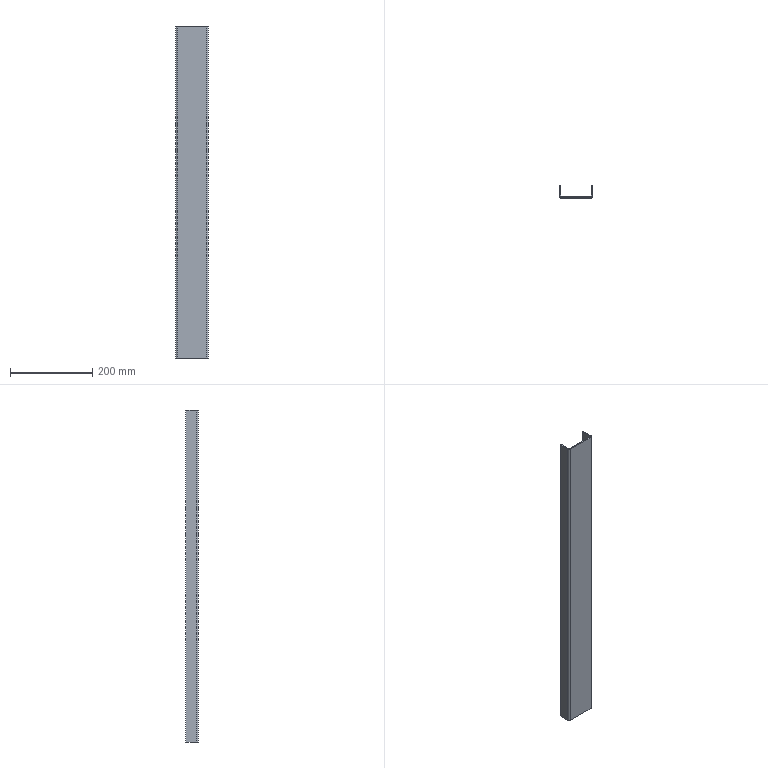Part | STEP file | Double-tube frame cross brace SGN-1-07 | 1 solid | 22 faces | box 80 x 30 x 807 mm | volume 318179 mm3 | plane 18 | cylinder 4 | commonest cylinder face diameters 3 x2 9 x2
STEP:
#1=CARTESIAN_POINT('',(0.,0.,0.));
#2=DIRECTION('',(0.,0.,1.));
#3=DIRECTION('',(1.,0.,0.));
#4=AXIS2_PLACEMENT_3D('',#1,#2,#3);
#5=CARTESIAN_POINT('',(35.5,-6.24,807.));
#6=VERTEX_POINT('',#5);
#7=CARTESIAN_POINT('',(35.5,-3.24,807.));
#8=VERTEX_POINT('',#7);
#9=CARTESIAN_POINT('',(35.5,-6.24,807.));
#10=DIRECTION('',(0.,1.,0.));
#11=VECTOR('',#10,1.);
#12=LINE('',#9,#11);
#13=CARTESIAN_POINT('',(35.5,-6.24,807.));
#14=DIRECTION('',(0.,0.,1.));
#15=DIRECTION('',(1.,0.,0.));
#16=AXIS2_PLACEMENT_3D('',#13,#14,#15);
#17=PLANE('',#16);
#18=CARTESIAN_POINT('',(0.,0.));
#19=DIRECTION('',(0.,1.));
#20=VECTOR('',#19,1.);
#21=LINE('',#18,#20);
#22=(GEOMETRIC_REPRESENTATION_CONTEXT(2)PARAMETRIC_REPRESENTATION_CONTEXT()REPRESENTATION_CONTEXT('',''));
#23=DEFINITIONAL_REPRESENTATION('',(#21),#22);
#24=PCURVE('',#17,#23);
#25=CARTESIAN_POINT('',(37.,-1.74,807.));
#26=DIRECTION('',(0.,0.,1.));
#27=DIRECTION('',(1.,0.,0.));
#28=AXIS2_PLACEMENT_3D('',#25,#26,#27);
#29=PLANE('',#28);
#30=CARTESIAN_POINT('',(-1.5,-4.5));
#31=DIRECTION('',(0.,1.));
#32=VECTOR('',#31,1.);
#33=LINE('',#30,#32);
#34=(GEOMETRIC_REPRESENTATION_CONTEXT(2)PARAMETRIC_REPRESENTATION_CONTEXT()REPRESENTATION_CONTEXT('',''));
#35=DEFINITIONAL_REPRESENTATION('',(#33),#34);
#36=PCURVE('',#29,#35);
#37=SURFACE_CURVE('',#12,(#24,#36),.PCURVE_S1.);
#38=EDGE_CURVE('',#6,#8,#37,.T.);
#39=ORIENTED_EDGE('',*,*,#38,.F.);
#40=CARTESIAN_POINT('',(40.,-1.74,807.));
#41=VERTEX_POINT('',#40);
#42=CARTESIAN_POINT('',(35.5,-1.74,807.));
#43=DIRECTION('',(0.,0.,-1.));
#44=DIRECTION('',(1.,0.,0.));
#45=AXIS2_PLACEMENT_3D('',#42,#43,#44);
#46=CIRCLE('',#45,4.5);
#47=CARTESIAN_POINT('',(4.5,4.5));
#48=CARTESIAN_POINT('',(4.5,-3.294));
#49=CARTESIAN_POINT('',(-2.25,0.6029));
#50=CARTESIAN_POINT('',(-9.,4.5));
#51=CARTESIAN_POINT('',(-2.25,8.397));
#52=CARTESIAN_POINT('',(4.5,12.294));
#53=CARTESIAN_POINT('',(4.5,4.5));
#54=(BOUNDED_CURVE()B_SPLINE_CURVE(2,(#47,#48,#49,#50,#51,#52,#53),.UNSPECIFIED.,.T.,.F.)B_SPLINE_CURVE_WITH_KNOTS((1,2,2,2,2,1),(-2.094,0.,2.094,4.189,6.283,8.378),.UNSPECIFIED.)CURVE()GEOMETRIC_REPRESENTATION_ITEM()RATIONAL_B_SPLINE_CURVE((1.,0.5,1.,0.5,1.,0.5,1.))REPRESENTATION_ITEM(''));
#55=(GEOMETRIC_REPRESENTATION_CONTEXT(2)PARAMETRIC_REPRESENTATION_CONTEXT()REPRESENTATION_CONTEXT('',''));
#56=DEFINITIONAL_REPRESENTATION('',(#54),#55);
#57=PCURVE('',#17,#56);
#58=CARTESIAN_POINT('',(35.5,-1.74,807.));
#59=DIRECTION('',(0.,0.,-1.));
#60=DIRECTION('',(-1.,0.,0.));
#61=AXIS2_PLACEMENT_3D('',#58,#59,#60);
#62=CYLINDRICAL_SURFACE('',#61,4.5);
#63=CARTESIAN_POINT('',(3.142,0.));
#64=DIRECTION('',(1.,0.));
#65=VECTOR('',#64,1.);
#66=LINE('',#63,#65);
#67=(GEOMETRIC_REPRESENTATION_CONTEXT(2)PARAMETRIC_REPRESENTATION_CONTEXT()REPRESENTATION_CONTEXT('',''));
#68=DEFINITIONAL_REPRESENTATION('',(#66),#67);
#69=PCURVE('',#62,#68);
#70=SURFACE_CURVE('',#46,(#57,#69),.PCURVE_S1.);
#71=EDGE_CURVE('',#41,#6,#70,.T.);
#72=ORIENTED_EDGE('',*,*,#71,.F.);
#73=CARTESIAN_POINT('',(37.,-1.74,807.));
#74=VERTEX_POINT('',#73);
#75=CARTESIAN_POINT('',(37.,-1.74,807.));
#76=DIRECTION('',(1.,0.,0.));
#77=VECTOR('',#76,1.);
#78=LINE('',#75,#77);
#79=CARTESIAN_POINT('',(1.5,4.5));
#80=DIRECTION('',(1.,0.));
#81=VECTOR('',#80,1.);
#82=LINE('',#79,#81);
#83=(GEOMETRIC_REPRESENTATION_CONTEXT(2)PARAMETRIC_REPRESENTATION_CONTEXT()REPRESENTATION_CONTEXT('',''));
#84=DEFINITIONAL_REPRESENTATION('',(#82),#83);
#85=PCURVE('',#17,#84);
#86=CARTESIAN_POINT('',(-35.5,-1.74,807.));
#87=DIRECTION('',(0.,0.,1.));
#88=DIRECTION('',(1.,0.,0.));
#89=AXIS2_PLACEMENT_3D('',#86,#87,#88);
#90=PLANE('',#89);
#91=CARTESIAN_POINT('',(72.5,0.));
#92=DIRECTION('',(1.,0.));
#93=VECTOR('',#92,1.);
#94=LINE('',#91,#93);
#95=(GEOMETRIC_REPRESENTATION_CONTEXT(2)PARAMETRIC_REPRESENTATION_CONTEXT()REPRESENTATION_CONTEXT('',''));
#96=DEFINITIONAL_REPRESENTATION('',(#94),#95);
#97=PCURVE('',#90,#96);
#98=SURFACE_CURVE('',#78,(#85,#97),.PCURVE_S1.);
#99=EDGE_CURVE('',#74,#41,#98,.T.);
#100=ORIENTED_EDGE('',*,*,#99,.F.);
#101=CARTESIAN_POINT('',(35.5,-1.74,807.));
#102=DIRECTION('',(0.,0.,-1.));
#103=DIRECTION('',(1.,0.,0.));
#104=AXIS2_PLACEMENT_3D('',#101,#102,#103);
#105=CIRCLE('',#104,1.5);
#106=CARTESIAN_POINT('',(1.5,4.5));
#107=CARTESIAN_POINT('',(1.5,1.902));
#108=CARTESIAN_POINT('',(-0.75,3.201));
#109=CARTESIAN_POINT('',(-3.,4.5));
#110=CARTESIAN_POINT('',(-0.75,5.799));
#111=CARTESIAN_POINT('',(1.5,7.098));
#112=CARTESIAN_POINT('',(1.5,4.5));
#113=(BOUNDED_CURVE()B_SPLINE_CURVE(2,(#106,#107,#108,#109,#110,#111,#112),.UNSPECIFIED.,.T.,.F.)B_SPLINE_CURVE_WITH_KNOTS((1,2,2,2,2,1),(-2.094,0.,2.094,4.189,6.283,8.378),.UNSPECIFIED.)CURVE()GEOMETRIC_REPRESENTATION_ITEM()RATIONAL_B_SPLINE_CURVE((1.,0.5,1.,0.5,1.,0.5,1.))REPRESENTATION_ITEM(''));
#114=(GEOMETRIC_REPRESENTATION_CONTEXT(2)PARAMETRIC_REPRESENTATION_CONTEXT()REPRESENTATION_CONTEXT('',''));
#115=DEFINITIONAL_REPRESENTATION('',(#113),#114);
#116=PCURVE('',#17,#115);
#117=CARTESIAN_POINT('',(35.5,-1.74,807.));
#118=DIRECTION('',(0.,0.,-1.));
#119=DIRECTION('',(-1.,0.,0.));
#120=AXIS2_PLACEMENT_3D('',#117,#118,#119);
#121=CYLINDRICAL_SURFACE('',#120,1.5);
#122=CARTESIAN_POINT('',(3.142,0.));
#123=DIRECTION('',(1.,0.));
#124=VECTOR('',#123,1.);
#125=LINE('',#122,#124);
#126=(GEOMETRIC_REPRESENTATION_CONTEXT(2)PARAMETRIC_REPRESENTATION_CONTEXT()REPRESENTATION_CONTEXT('',''));
#127=DEFINITIONAL_REPRESENTATION('',(#125),#126);
#128=PCURVE('',#121,#127);
#129=SURFACE_CURVE('',#105,(#116,#128),.PCURVE_S1.);
#130=EDGE_CURVE('',#74,#8,#129,.T.);
#131=ORIENTED_EDGE('',*,*,#130,.T.);
#132=EDGE_LOOP('',(#39,#72,#100,#131));
#133=FACE_BOUND('',#132,.T.);
#134=ADVANCED_FACE('',(#133),#17,.T.);
#135=CARTESIAN_POINT('',(-35.5,-6.24,807.));
#136=VERTEX_POINT('',#135);
#137=CARTESIAN_POINT('',(-40.,-6.24,807.));
#138=DIRECTION('',(-1.,0.,0.));
#139=VECTOR('',#138,1.);
#140=LINE('',#137,#139);
#141=CARTESIAN_POINT('',(-77.,-4.5));
#142=DIRECTION('',(-1.,0.));
#143=VECTOR('',#142,1.);
#144=LINE('',#141,#143);
#145=(GEOMETRIC_REPRESENTATION_CONTEXT(2)PARAMETRIC_REPRESENTATION_CONTEXT()REPRESENTATION_CONTEXT('',''));
#146=DEFINITIONAL_REPRESENTATION('',(#144),#145);
#147=PCURVE('',#29,#146);
#148=CARTESIAN_POINT('',(-40.,-6.24,807.));
#149=DIRECTION('',(0.,-1.,0.));
#150=DIRECTION('',(0.,0.,-1.));
#151=AXIS2_PLACEMENT_3D('',#148,#149,#150);
#152=PLANE('',#151);
#153=CARTESIAN_POINT('',(0.,0.));
#154=DIRECTION('',(0.,-1.));
#155=VECTOR('',#154,1.);
#156=LINE('',#153,#155);
#157=(GEOMETRIC_REPRESENTATION_CONTEXT(2)PARAMETRIC_REPRESENTATION_CONTEXT()REPRESENTATION_CONTEXT('',''));
#158=DEFINITIONAL_REPRESENTATION('',(#156),#157);
#159=PCURVE('',#152,#158);
#160=SURFACE_CURVE('',#140,(#147,#159),.PCURVE_S1.);
#161=EDGE_CURVE('',#6,#136,#160,.T.);
#162=ORIENTED_EDGE('',*,*,#161,.F.);
#163=ORIENTED_EDGE('',*,*,#38,.T.);
#164=CARTESIAN_POINT('',(-35.5,-3.24,807.));
#165=VERTEX_POINT('',#164);
#166=CARTESIAN_POINT('',(-40.,-3.24,807.));
#167=DIRECTION('',(-1.,0.,0.));
#168=VECTOR('',#167,1.);
#169=LINE('',#166,#168);
#170=CARTESIAN_POINT('',(-77.,-1.5));
#171=DIRECTION('',(-1.,0.));
#172=VECTOR('',#171,1.);
#173=LINE('',#170,#172);
#174=(GEOMETRIC_REPRESENTATION_CONTEXT(2)PARAMETRIC_REPRESENTATION_CONTEXT()REPRESENTATION_CONTEXT('',''));
#175=DEFINITIONAL_REPRESENTATION('',(#173),#174);
#176=PCURVE('',#29,#175);
#177=CARTESIAN_POINT('',(-40.,-3.24,807.));
#178=DIRECTION('',(0.,-1.,0.));
#179=DIRECTION('',(0.,0.,-1.));
#180=AXIS2_PLACEMENT_3D('',#177,#178,#179);
#181=PLANE('',#180);
#182=CARTESIAN_POINT('',(0.,0.));
#183=DIRECTION('',(0.,-1.));
#184=VECTOR('',#183,1.);
#185=LINE('',#182,#184);
#186=(GEOMETRIC_REPRESENTATION_CONTEXT(2)PARAMETRIC_REPRESENTATION_CONTEXT()REPRESENTATION_CONTEXT('',''));
#187=DEFINITIONAL_REPRESENTATION('',(#185),#186);
#188=PCURVE('',#181,#187);
#189=SURFACE_CURVE('',#169,(#176,#188),.PCURVE_S1.);
#190=EDGE_CURVE('',#8,#165,#189,.T.);
#191=ORIENTED_EDGE('',*,*,#190,.T.);
#192=CARTESIAN_POINT('',(-35.5,-3.24,807.));
#193=DIRECTION('',(0.,-1.,0.));
#194=VECTOR('',#193,1.);
#195=LINE('',#192,#194);
#196=CARTESIAN_POINT('',(-72.5,-1.5));
#197=DIRECTION('',(0.,-1.));
#198=VECTOR('',#197,1.);
#199=LINE('',#196,#198);
#200=(GEOMETRIC_REPRESENTATION_CONTEXT(2)PARAMETRIC_REPRESENTATION_CONTEXT()REPRESENTATION_CONTEXT('',''));
#201=DEFINITIONAL_REPRESENTATION('',(#199),#200);
#202=PCURVE('',#29,#201);
#203=CARTESIAN_POINT('',(-40.,-1.74,807.));
#204=DIRECTION('',(0.,0.,1.));
#205=DIRECTION('',(1.,0.,0.));
#206=AXIS2_PLACEMENT_3D('',#203,#204,#205);
#207=PLANE('',#206);
#208=CARTESIAN_POINT('',(4.5,-1.5));
#209=DIRECTION('',(0.,-1.));
#210=VECTOR('',#209,1.);
#211=LINE('',#208,#210);
#212=(GEOMETRIC_REPRESENTATION_CONTEXT(2)PARAMETRIC_REPRESENTATION_CONTEXT()REPRESENTATION_CONTEXT('',''));
#213=DEFINITIONAL_REPRESENTATION('',(#211),#212);
#214=PCURVE('',#207,#213);
#215=SURFACE_CURVE('',#195,(#202,#214),.PCURVE_S1.);
#216=EDGE_CURVE('',#165,#136,#215,.T.);
#217=ORIENTED_EDGE('',*,*,#216,.T.);
#218=EDGE_LOOP('',(#162,#163,#191,#217));
#219=FACE_BOUND('',#218,.T.);
#220=ADVANCED_FACE('',(#219),#29,.T.);
#221=CARTESIAN_POINT('',(40.,-1.74,0.));
#222=VERTEX_POINT('',#221);
#223=CARTESIAN_POINT('',(37.,-1.74,0.));
#224=VERTEX_POINT('',#223);
#225=CARTESIAN_POINT('',(40.,-1.74,0.));
#226=DIRECTION('',(-1.,0.,0.));
#227=VECTOR('',#226,1.);
#228=LINE('',#225,#227);
#229=CARTESIAN_POINT('',(40.,-1.74,0.));
#230=DIRECTION('',(0.,0.,-1.));
#231=DIRECTION('',(-1.,0.,0.));
#232=AXIS2_PLACEMENT_3D('',#229,#230,#231);
#233=PLANE('',#232);
#234=CARTESIAN_POINT('',(0.,0.));
#235=DIRECTION('',(1.,0.));
#236=VECTOR('',#235,1.);
#237=LINE('',#234,#236);
#238=(GEOMETRIC_REPRESENTATION_CONTEXT(2)PARAMETRIC_REPRESENTATION_CONTEXT()REPRESENTATION_CONTEXT('',''));
#239=DEFINITIONAL_REPRESENTATION('',(#237),#238);
#240=PCURVE('',#233,#239);
#241=CARTESIAN_POINT('',(35.5,-3.24,0.));
#242=DIRECTION('',(0.,0.,-1.));
#243=DIRECTION('',(-1.,0.,0.));
#244=AXIS2_PLACEMENT_3D('',#241,#242,#243);
#245=PLANE('',#244);
#246=CARTESIAN_POINT('',(-4.5,1.5));
#247=DIRECTION('',(1.,0.));
#248=VECTOR('',#247,1.);
#249=LINE('',#246,#248);
#250=(GEOMETRIC_REPRESENTATION_CONTEXT(2)PARAMETRIC_REPRESENTATION_CONTEXT()REPRESENTATION_CONTEXT('',''));
#251=DEFINITIONAL_REPRESENTATION('',(#249),#250);
#252=PCURVE('',#245,#251);
#253=SURFACE_CURVE('',#228,(#240,#252),.PCURVE_S1.);
#254=EDGE_CURVE('',#222,#224,#253,.T.);
#255=ORIENTED_EDGE('',*,*,#254,.F.);
#256=CARTESIAN_POINT('',(35.5,-6.24,0.));
#257=VERTEX_POINT('',#256);
#258=CARTESIAN_POINT('',(35.5,-1.74,0.));
#259=DIRECTION('',(0.,0.,-1.));
#260=DIRECTION('',(1.,0.,0.));
#261=AXIS2_PLACEMENT_3D('',#258,#259,#260);
#262=CIRCLE('',#261,4.5);
#263=CARTESIAN_POINT('',(4.5,0.));
#264=DIRECTION('',(-1.,0.));
#265=AXIS2_PLACEMENT_2D('',#263,#264);
#266=CIRCLE('',#265,4.5);
#267=(GEOMETRIC_REPRESENTATION_CONTEXT(2)PARAMETRIC_REPRESENTATION_CONTEXT()REPRESENTATION_CONTEXT('',''));
#268=DEFINITIONAL_REPRESENTATION('',(#266),#267);
#269=PCURVE('',#233,#268);
#270=CARTESIAN_POINT('',(3.142,807.));
#271=DIRECTION('',(1.,0.));
#272=VECTOR('',#271,1.);
#273=LINE('',#270,#272);
#274=(GEOMETRIC_REPRESENTATION_CONTEXT(2)PARAMETRIC_REPRESENTATION_CONTEXT()REPRESENTATION_CONTEXT('',''));
#275=DEFINITIONAL_REPRESENTATION('',(#273),#274);
#276=PCURVE('',#62,#275);
#277=SURFACE_CURVE('',#262,(#269,#276),.PCURVE_S1.);
#278=EDGE_CURVE('',#222,#257,#277,.T.);
#279=ORIENTED_EDGE('',*,*,#278,.T.);
#280=CARTESIAN_POINT('',(35.5,-3.24,0.));
#281=VERTEX_POINT('',#280);
#282=CARTESIAN_POINT('',(35.5,-3.24,0.));
#283=DIRECTION('',(0.,-1.,0.));
#284=VECTOR('',#283,1.);
#285=LINE('',#282,#284);
#286=CARTESIAN_POINT('',(4.5,-1.5));
#287=DIRECTION('',(0.,-1.));
#288=VECTOR('',#287,1.);
#289=LINE('',#286,#288);
#290=(GEOMETRIC_REPRESENTATION_CONTEXT(2)PARAMETRIC_REPRESENTATION_CONTEXT()REPRESENTATION_CONTEXT('',''));
#291=DEFINITIONAL_REPRESENTATION('',(#289),#290);
#292=PCURVE('',#233,#291);
#293=CARTESIAN_POINT('',(-37.,-1.74,0.));
#294=DIRECTION('',(0.,0.,-1.));
#295=DIRECTION('',(-1.,0.,0.));
#296=AXIS2_PLACEMENT_3D('',#293,#294,#295);
#297=PLANE('',#296);
#298=CARTESIAN_POINT('',(-72.5,-1.5));
#299=DIRECTION('',(0.,-1.));
#300=VECTOR('',#299,1.);
#301=LINE('',#298,#300);
#302=(GEOMETRIC_REPRESENTATION_CONTEXT(2)PARAMETRIC_REPRESENTATION_CONTEXT()REPRESENTATION_CONTEXT('',''));
#303=DEFINITIONAL_REPRESENTATION('',(#301),#302);
#304=PCURVE('',#297,#303);
#305=SURFACE_CURVE('',#285,(#292,#304),.PCURVE_S1.);
#306=EDGE_CURVE('',#281,#257,#305,.T.);
#307=ORIENTED_EDGE('',*,*,#306,.F.);
#308=CARTESIAN_POINT('',(35.5,-1.74,0.));
#309=DIRECTION('',(0.,0.,-1.));
#310=DIRECTION('',(1.,0.,0.));
#311=AXIS2_PLACEMENT_3D('',#308,#309,#310);
#312=CIRCLE('',#311,1.5);
#313=CARTESIAN_POINT('',(4.5,0.));
#314=DIRECTION('',(-1.,0.));
#315=AXIS2_PLACEMENT_2D('',#313,#314);
#316=CIRCLE('',#315,1.5);
#317=(GEOMETRIC_REPRESENTATION_CONTEXT(2)PARAMETRIC_REPRESENTATION_CONTEXT()REPRESENTATION_CONTEXT('',''));
#318=DEFINITIONAL_REPRESENTATION('',(#316),#317);
#319=PCURVE('',#233,#318);
#320=CARTESIAN_POINT('',(3.142,807.));
#321=DIRECTION('',(1.,0.));
#322=VECTOR('',#321,1.);
#323=LINE('',#320,#322);
#324=(GEOMETRIC_REPRESENTATION_CONTEXT(2)PARAMETRIC_REPRESENTATION_CONTEXT()REPRESENTATION_CONTEXT('',''));
#325=DEFINITIONAL_REPRESENTATION('',(#323),#324);
#326=PCURVE('',#121,#325);
#327=SURFACE_CURVE('',#312,(#319,#326),.PCURVE_S1.);
#328=EDGE_CURVE('',#224,#281,#327,.T.);
#329=ORIENTED_EDGE('',*,*,#328,.F.);
#330=EDGE_LOOP('',(#255,#279,#307,#329));
#331=FACE_BOUND('',#330,.T.);
#332=ADVANCED_FACE('',(#331),#233,.T.);
#333=CARTESIAN_POINT('',(40.,23.76,0.));
#334=VERTEX_POINT('',#333);
#335=CARTESIAN_POINT('',(40.,-6.24,0.));
#336=DIRECTION('',(0.,-1.,0.));
#337=VECTOR('',#336,1.);
#338=LINE('',#335,#337);
#339=CARTESIAN_POINT('',(-4.5,-3.));
#340=DIRECTION('',(0.,-1.));
#341=VECTOR('',#340,1.);
#342=LINE('',#339,#341);
#343=(GEOMETRIC_REPRESENTATION_CONTEXT(2)PARAMETRIC_REPRESENTATION_CONTEXT()REPRESENTATION_CONTEXT('',''));
#344=DEFINITIONAL_REPRESENTATION('',(#342),#343);
#345=PCURVE('',#245,#344);
#346=CARTESIAN_POINT('',(40.,-6.24,807.));
#347=DIRECTION('',(1.,0.,0.));
#348=DIRECTION('',(0.,0.,-1.));
#349=AXIS2_PLACEMENT_3D('',#346,#347,#348);
#350=PLANE('',#349);
#351=CARTESIAN_POINT('',(807.,0.));
#352=DIRECTION('',(0.,-1.));
#353=VECTOR('',#352,1.);
#354=LINE('',#351,#353);
#355=(GEOMETRIC_REPRESENTATION_CONTEXT(2)PARAMETRIC_REPRESENTATION_CONTEXT()REPRESENTATION_CONTEXT('',''));
#356=DEFINITIONAL_REPRESENTATION('',(#354),#355);
#357=PCURVE('',#350,#356);
#358=SURFACE_CURVE('',#338,(#345,#357),.PCURVE_S1.);
#359=EDGE_CURVE('',#334,#222,#358,.T.);
#360=ORIENTED_EDGE('',*,*,#359,.T.);
#361=ORIENTED_EDGE('',*,*,#254,.T.);
#362=CARTESIAN_POINT('',(37.,23.76,0.));
#363=VERTEX_POINT('',#362);
#364=CARTESIAN_POINT('',(37.,-6.24,0.));
#365=DIRECTION('',(0.,-1.,0.));
#366=VECTOR('',#365,1.);
#367=LINE('',#364,#366);
#368=CARTESIAN_POINT('',(-1.5,-3.));
#369=DIRECTION('',(0.,-1.));
#370=VECTOR('',#369,1.);
#371=LINE('',#368,#370);
#372=(GEOMETRIC_REPRESENTATION_CONTEXT(2)PARAMETRIC_REPRESENTATION_CONTEXT()REPRESENTATION_CONTEXT('',''));
#373=DEFINITIONAL_REPRESENTATION('',(#371),#372);
#374=PCURVE('',#245,#373);
#375=CARTESIAN_POINT('',(37.,-6.24,807.));
#376=DIRECTION('',(1.,0.,0.));
#377=DIRECTION('',(0.,0.,-1.));
#378=AXIS2_PLACEMENT_3D('',#375,#376,#377);
#379=PLANE('',#378);
#380=CARTESIAN_POINT('',(807.,0.));
#381=DIRECTION('',(0.,-1.));
#382=VECTOR('',#381,1.);
#383=LINE('',#380,#382);
#384=(GEOMETRIC_REPRESENTATION_CONTEXT(2)PARAMETRIC_REPRESENTATION_CONTEXT()REPRESENTATION_CONTEXT('',''));
#385=DEFINITIONAL_REPRESENTATION('',(#383),#384);
#386=PCURVE('',#379,#385);
#387=SURFACE_CURVE('',#367,(#374,#386),.PCURVE_S1.);
#388=EDGE_CURVE('',#363,#224,#387,.T.);
#389=ORIENTED_EDGE('',*,*,#388,.F.);
#390=CARTESIAN_POINT('',(37.,23.76,0.));
#391=DIRECTION('',(1.,0.,0.));
#392=VECTOR('',#391,1.);
#393=LINE('',#390,#392);
#394=CARTESIAN_POINT('',(-1.5,27.));
#395=DIRECTION('',(-1.,0.));
#396=VECTOR('',#395,1.);
#397=LINE('',#394,#396);
#398=(GEOMETRIC_REPRESENTATION_CONTEXT(2)PARAMETRIC_REPRESENTATION_CONTEXT()REPRESENTATION_CONTEXT('',''));
#399=DEFINITIONAL_REPRESENTATION('',(#397),#398);
#400=PCURVE('',#245,#399);
#401=CARTESIAN_POINT('',(37.,23.76,807.));
#402=DIRECTION('',(0.,1.,0.));
#403=DIRECTION('',(0.,0.,1.));
#404=AXIS2_PLACEMENT_3D('',#401,#402,#403);
#405=PLANE('',#404);
#406=CARTESIAN_POINT('',(-807.,0.));
#407=DIRECTION('',(0.,1.));
#408=VECTOR('',#407,1.);
#409=LINE('',#406,#408);
#410=(GEOMETRIC_REPRESENTATION_CONTEXT(2)PARAMETRIC_REPRESENTATION_CONTEXT()REPRESENTATION_CONTEXT('',''));
#411=DEFINITIONAL_REPRESENTATION('',(#409),#410);
#412=PCURVE('',#405,#411);
#413=SURFACE_CURVE('',#393,(#400,#412),.PCURVE_S1.);
#414=EDGE_CURVE('',#363,#334,#413,.T.);
#415=ORIENTED_EDGE('',*,*,#414,.T.);
#416=EDGE_LOOP('',(#360,#361,#389,#415));
#417=FACE_BOUND('',#416,.T.);
#418=ADVANCED_FACE('',(#417),#245,.T.);
#419=CARTESIAN_POINT('',(-40.,-1.74,807.));
#420=VERTEX_POINT('',#419);
#421=CARTESIAN_POINT('',(-37.,-1.74,807.));
#422=VERTEX_POINT('',#421);
#423=CARTESIAN_POINT('',(-40.,-1.74,807.));
#424=DIRECTION('',(1.,0.,0.));
#425=VECTOR('',#424,1.);
#426=LINE('',#423,#425);
#427=CARTESIAN_POINT('',(0.,0.));
#428=DIRECTION('',(1.,0.));
#429=VECTOR('',#428,1.);
#430=LINE('',#427,#429);
#431=(GEOMETRIC_REPRESENTATION_CONTEXT(2)PARAMETRIC_REPRESENTATION_CONTEXT()REPRESENTATION_CONTEXT('',''));
#432=DEFINITIONAL_REPRESENTATION('',(#430),#431);
#433=PCURVE('',#207,#432);
#434=CARTESIAN_POINT('',(-35.5,-3.24,807.));
#435=DIRECTION('',(0.,0.,1.));
#436=DIRECTION('',(1.,0.,0.));
#437=AXIS2_PLACEMENT_3D('',#434,#435,#436);
#438=PLANE('',#437);
#439=CARTESIAN_POINT('',(-4.5,1.5));
#440=DIRECTION('',(1.,0.));
#441=VECTOR('',#440,1.);
#442=LINE('',#439,#441);
#443=(GEOMETRIC_REPRESENTATION_CONTEXT(2)PARAMETRIC_REPRESENTATION_CONTEXT()REPRESENTATION_CONTEXT('',''));
#444=DEFINITIONAL_REPRESENTATION('',(#442),#443);
#445=PCURVE('',#438,#444);
#446=SURFACE_CURVE('',#426,(#433,#445),.PCURVE_S1.);
#447=EDGE_CURVE('',#420,#422,#446,.T.);
#448=ORIENTED_EDGE('',*,*,#447,.F.);
#449=CARTESIAN_POINT('',(-35.5,-1.74,807.));
#450=DIRECTION('',(0.,0.,-1.));
#451=DIRECTION('',(1.,0.,0.));
#452=AXIS2_PLACEMENT_3D('',#449,#450,#451);
#453=CIRCLE('',#452,4.5);
#454=CARTESIAN_POINT('',(9.,0.));
#455=CARTESIAN_POINT('',(9.,-7.794));
#456=CARTESIAN_POINT('',(2.25,-3.897));
#457=CARTESIAN_POINT('',(-4.5,0.));
#458=CARTESIAN_POINT('',(2.25,3.897));
#459=CARTESIAN_POINT('',(9.,7.794));
#460=CARTESIAN_POINT('',(9.,0.));
#461=(BOUNDED_CURVE()B_SPLINE_CURVE(2,(#454,#455,#456,#457,#458,#459,#460),.UNSPECIFIED.,.T.,.F.)B_SPLINE_CURVE_WITH_KNOTS((1,2,2,2,2,1),(-2.094,0.,2.094,4.189,6.283,8.378),.UNSPECIFIED.)CURVE()GEOMETRIC_REPRESENTATION_ITEM()RATIONAL_B_SPLINE_CURVE((1.,0.5,1.,0.5,1.,0.5,1.))REPRESENTATION_ITEM(''));
#462=(GEOMETRIC_REPRESENTATION_CONTEXT(2)PARAMETRIC_REPRESENTATION_CONTEXT()REPRESENTATION_CONTEXT('',''));
#463=DEFINITIONAL_REPRESENTATION('',(#461),#462);
#464=PCURVE('',#207,#463);
#465=CARTESIAN_POINT('',(-35.5,-1.74,807.));
#466=DIRECTION('',(0.,0.,-1.));
#467=DIRECTION('',(-1.,0.,0.));
#468=AXIS2_PLACEMENT_3D('',#465,#466,#467);
#469=CYLINDRICAL_SURFACE('',#468,4.5);
#470=CARTESIAN_POINT('',(3.142,0.));
#471=DIRECTION('',(1.,0.));
#472=VECTOR('',#471,1.);
#473=LINE('',#470,#472);
#474=(GEOMETRIC_REPRESENTATION_CONTEXT(2)PARAMETRIC_REPRESENTATION_CONTEXT()REPRESENTATION_CONTEXT('',''));
#475=DEFINITIONAL_REPRESENTATION('',(#473),#474);
#476=PCURVE('',#469,#475);
#477=SURFACE_CURVE('',#453,(#464,#476),.PCURVE_S1.);
#478=EDGE_CURVE('',#136,#420,#477,.T.);
#479=ORIENTED_EDGE('',*,*,#478,.F.);
#480=ORIENTED_EDGE('',*,*,#216,.F.);
#481=CARTESIAN_POINT('',(-35.5,-1.74,807.));
#482=DIRECTION('',(0.,0.,-1.));
#483=DIRECTION('',(1.,0.,0.));
#484=AXIS2_PLACEMENT_3D('',#481,#482,#483);
#485=CIRCLE('',#484,1.5);
#486=CARTESIAN_POINT('',(6.,0.));
#487=CARTESIAN_POINT('',(6.,-2.598));
#488=CARTESIAN_POINT('',(3.75,-1.299));
#489=CARTESIAN_POINT('',(1.5,0.));
#490=CARTESIAN_POINT('',(3.75,1.299));
#491=CARTESIAN_POINT('',(6.,2.598));
#492=CARTESIAN_POINT('',(6.,0.));
#493=(BOUNDED_CURVE()B_SPLINE_CURVE(2,(#486,#487,#488,#489,#490,#491,#492),.UNSPECIFIED.,.T.,.F.)B_SPLINE_CURVE_WITH_KNOTS((1,2,2,2,2,1),(-2.094,0.,2.094,4.189,6.283,8.378),.UNSPECIFIED.)CURVE()GEOMETRIC_REPRESENTATION_ITEM()RATIONAL_B_SPLINE_CURVE((1.,0.5,1.,0.5,1.,0.5,1.))REPRESENTATION_ITEM(''));
#494=(GEOMETRIC_REPRESENTATION_CONTEXT(2)PARAMETRIC_REPRESENTATION_CONTEXT()REPRESENTATION_CONTEXT('',''));
#495=DEFINITIONAL_REPRESENTATION('',(#493),#494);
#496=PCURVE('',#207,#495);
#497=CARTESIAN_POINT('',(-35.5,-1.74,807.));
#498=DIRECTION('',(0.,0.,-1.));
#499=DIRECTION('',(-1.,0.,0.));
#500=AXIS2_PLACEMENT_3D('',#497,#498,#499);
#501=CYLINDRICAL_SURFACE('',#500,1.5);
#502=CARTESIAN_POINT('',(3.142,0.));
#503=DIRECTION('',(1.,0.));
#504=VECTOR('',#503,1.);
#505=LINE('',#502,#504);
#506=(GEOMETRIC_REPRESENTATION_CONTEXT(2)PARAMETRIC_REPRESENTATION_CONTEXT()REPRESENTATION_CONTEXT('',''));
#507=DEFINITIONAL_REPRESENTATION('',(#505),#506);
#508=PCURVE('',#501,#507);
#509=SURFACE_CURVE('',#485,(#496,#508),.PCURVE_S1.);
#510=EDGE_CURVE('',#165,#422,#509,.T.);
#511=ORIENTED_EDGE('',*,*,#510,.T.);
#512=EDGE_LOOP('',(#448,#479,#480,#511));
#513=FACE_BOUND('',#512,.T.);
#514=ADVANCED_FACE('',(#513),#207,.T.);
#515=CARTESIAN_POINT('',(-40.,23.76,807.));
#516=VERTEX_POINT('',#515);
#517=CARTESIAN_POINT('',(-40.,-6.24,807.));
#518=DIRECTION('',(0.,1.,0.));
#519=VECTOR('',#518,1.);
#520=LINE('',#517,#519);
#521=CARTESIAN_POINT('',(-4.5,-3.));
#522=DIRECTION('',(0.,1.));
#523=VECTOR('',#522,1.);
#524=LINE('',#521,#523);
#525=(GEOMETRIC_REPRESENTATION_CONTEXT(2)PARAMETRIC_REPRESENTATION_CONTEXT()REPRESENTATION_CONTEXT('',''));
#526=DEFINITIONAL_REPRESENTATION('',(#524),#525);
#527=PCURVE('',#438,#526);
#528=CARTESIAN_POINT('',(-40.,-6.24,807.));
#529=DIRECTION('',(-1.,0.,0.));
#530=DIRECTION('',(0.,0.,1.));
#531=AXIS2_PLACEMENT_3D('',#528,#529,#530);
#532=PLANE('',#531);
#533=CARTESIAN_POINT('',(0.,0.));
#534=DIRECTION('',(0.,1.));
#535=VECTOR('',#534,1.);
#536=LINE('',#533,#535);
#537=(GEOMETRIC_REPRESENTATION_CONTEXT(2)PARAMETRIC_REPRESENTATION_CONTEXT()REPRESENTATION_CONTEXT('',''));
#538=DEFINITIONAL_REPRESENTATION('',(#536),#537);
#539=PCURVE('',#532,#538);
#540=SURFACE_CURVE('',#520,(#527,#539),.PCURVE_S1.);
#541=EDGE_CURVE('',#420,#516,#540,.T.);
#542=ORIENTED_EDGE('',*,*,#541,.F.);
#543=ORIENTED_EDGE('',*,*,#447,.T.);
#544=CARTESIAN_POINT('',(-37.,23.76,807.));
#545=VERTEX_POINT('',#544);
#546=CARTESIAN_POINT('',(-37.,-6.24,807.));
#547=DIRECTION('',(0.,1.,0.));
#548=VECTOR('',#547,1.);
#549=LINE('',#546,#548);
#550=CARTESIAN_POINT('',(-1.5,-3.));
#551=DIRECTION('',(0.,1.));
#552=VECTOR('',#551,1.);
#553=LINE('',#550,#552);
#554=(GEOMETRIC_REPRESENTATION_CONTEXT(2)PARAMETRIC_REPRESENTATION_CONTEXT()REPRESENTATION_CONTEXT('',''));
#555=DEFINITIONAL_REPRESENTATION('',(#553),#554);
#556=PCURVE('',#438,#555);
#557=CARTESIAN_POINT('',(-37.,-6.24,807.));
#558=DIRECTION('',(-1.,0.,0.));
#559=DIRECTION('',(0.,0.,1.));
#560=AXIS2_PLACEMENT_3D('',#557,#558,#559);
#561=PLANE('',#560);
#562=CARTESIAN_POINT('',(0.,0.));
#563=DIRECTION('',(0.,1.));
#564=VECTOR('',#563,1.);
#565=LINE('',#562,#564);
#566=(GEOMETRIC_REPRESENTATION_CONTEXT(2)PARAMETRIC_REPRESENTATION_CONTEXT()REPRESENTATION_CONTEXT('',''));
#567=DEFINITIONAL_REPRESENTATION('',(#565),#566);
#568=PCURVE('',#561,#567);
#569=SURFACE_CURVE('',#549,(#556,#568),.PCURVE_S1.);
#570=EDGE_CURVE('',#422,#545,#569,.T.);
#571=ORIENTED_EDGE('',*,*,#570,.T.);
#572=CARTESIAN_POINT('',(-40.,23.76,807.));
#573=DIRECTION('',(1.,0.,0.));
#574=VECTOR('',#573,1.);
#575=LINE('',#572,#574);
#576=CARTESIAN_POINT('',(-4.5,27.));
#577=DIRECTION('',(1.,0.));
#578=VECTOR('',#577,1.);
#579=LINE('',#576,#578);
#580=(GEOMETRIC_REPRESENTATION_CONTEXT(2)PARAMETRIC_REPRESENTATION_CONTEXT()REPRESENTATION_CONTEXT('',''));
#581=DEFINITIONAL_REPRESENTATION('',(#579),#580);
#582=PCURVE('',#438,#581);
#583=CARTESIAN_POINT('',(-40.,23.76,807.));
#584=DIRECTION('',(0.,1.,0.));
#585=DIRECTION('',(0.,0.,1.));
#586=AXIS2_PLACEMENT_3D('',#583,#584,#585);
#587=PLANE('',#586);
#588=CARTESIAN_POINT('',(0.,0.));
#589=DIRECTION('',(0.,1.));
#590=VECTOR('',#589,1.);
#591=LINE('',#588,#590);
#592=(GEOMETRIC_REPRESENTATION_CONTEXT(2)PARAMETRIC_REPRESENTATION_CONTEXT()REPRESENTATION_CONTEXT('',''));
#593=DEFINITIONAL_REPRESENTATION('',(#591),#592);
#594=PCURVE('',#587,#593);
#595=SURFACE_CURVE('',#575,(#582,#594),.PCURVE_S1.);
#596=EDGE_CURVE('',#516,#545,#595,.T.);
#597=ORIENTED_EDGE('',*,*,#596,.F.);
#598=EDGE_LOOP('',(#542,#543,#571,#597));
#599=FACE_BOUND('',#598,.T.);
#600=ADVANCED_FACE('',(#599),#438,.T.);
#601=CARTESIAN_POINT('',(-35.5,-6.24,0.));
#602=VERTEX_POINT('',#601);
#603=CARTESIAN_POINT('',(-35.5,-3.24,0.));
#604=VERTEX_POINT('',#603);
#605=CARTESIAN_POINT('',(-35.5,-6.24,0.));
#606=DIRECTION('',(0.,1.,0.));
#607=VECTOR('',#606,1.);
#608=LINE('',#605,#607);
#609=CARTESIAN_POINT('',(-35.5,-6.24,0.));
#610=DIRECTION('',(0.,0.,-1.));
#611=DIRECTION('',(-1.,0.,0.));
#612=AXIS2_PLACEMENT_3D('',#609,#610,#611);
#613=PLANE('',#612);
#614=CARTESIAN_POINT('',(0.,0.));
#615=DIRECTION('',(0.,1.));
#616=VECTOR('',#615,1.);
#617=LINE('',#614,#616);
#618=(GEOMETRIC_REPRESENTATION_CONTEXT(2)PARAMETRIC_REPRESENTATION_CONTEXT()REPRESENTATION_CONTEXT('',''));
#619=DEFINITIONAL_REPRESENTATION('',(#617),#618);
#620=PCURVE('',#613,#619);
#621=CARTESIAN_POINT('',(-1.5,-4.5));
#622=DIRECTION('',(0.,1.));
#623=VECTOR('',#622,1.);
#624=LINE('',#621,#623);
#625=(GEOMETRIC_REPRESENTATION_CONTEXT(2)PARAMETRIC_REPRESENTATION_CONTEXT()REPRESENTATION_CONTEXT('',''));
#626=DEFINITIONAL_REPRESENTATION('',(#624),#625);
#627=PCURVE('',#297,#626);
#628=SURFACE_CURVE('',#608,(#620,#627),.PCURVE_S1.);
#629=EDGE_CURVE('',#602,#604,#628,.T.);
#630=ORIENTED_EDGE('',*,*,#629,.F.);
#631=CARTESIAN_POINT('',(-40.,-1.74,0.));
#632=VERTEX_POINT('',#631);
#633=CARTESIAN_POINT('',(-35.5,-1.74,0.));
#634=DIRECTION('',(0.,0.,-1.));
#635=DIRECTION('',(1.,0.,0.));
#636=AXIS2_PLACEMENT_3D('',#633,#634,#635);
#637=CIRCLE('',#636,4.5);
#638=CARTESIAN_POINT('',(0.,4.5));
#639=DIRECTION('',(-1.,0.));
#640=AXIS2_PLACEMENT_2D('',#638,#639);
#641=CIRCLE('',#640,4.5);
#642=(GEOMETRIC_REPRESENTATION_CONTEXT(2)PARAMETRIC_REPRESENTATION_CONTEXT()REPRESENTATION_CONTEXT('',''));
#643=DEFINITIONAL_REPRESENTATION('',(#641),#642);
#644=PCURVE('',#613,#643);
#645=CARTESIAN_POINT('',(3.142,807.));
#646=DIRECTION('',(1.,0.));
#647=VECTOR('',#646,1.);
#648=LINE('',#645,#647);
#649=(GEOMETRIC_REPRESENTATION_CONTEXT(2)PARAMETRIC_REPRESENTATION_CONTEXT()REPRESENTATION_CONTEXT('',''));
#650=DEFINITIONAL_REPRESENTATION('',(#648),#649);
#651=PCURVE('',#469,#650);
#652=SURFACE_CURVE('',#637,(#644,#651),.PCURVE_S1.);
#653=EDGE_CURVE('',#602,#632,#652,.T.);
#654=ORIENTED_EDGE('',*,*,#653,.T.);
#655=CARTESIAN_POINT('',(-37.,-1.74,0.));
#656=VERTEX_POINT('',#655);
#657=CARTESIAN_POINT('',(-37.,-1.74,0.));
#658=DIRECTION('',(-1.,0.,0.));
#659=VECTOR('',#658,1.);
#660=LINE('',#657,#659);
#661=CARTESIAN_POINT('',(1.5,4.5));
#662=DIRECTION('',(1.,0.));
#663=VECTOR('',#662,1.);
#664=LINE('',#661,#663);
#665=(GEOMETRIC_REPRESENTATION_CONTEXT(2)PARAMETRIC_REPRESENTATION_CONTEXT()REPRESENTATION_CONTEXT('',''));
#666=DEFINITIONAL_REPRESENTATION('',(#664),#665);
#667=PCURVE('',#613,#666);
#668=CARTESIAN_POINT('',(-35.5,-1.74,0.));
#669=DIRECTION('',(0.,0.,1.));
#670=DIRECTION('',(1.,0.,0.));
#671=AXIS2_PLACEMENT_3D('',#668,#669,#670);
#672=PLANE('',#671);
#673=CARTESIAN_POINT('',(-1.5,0.));
#674=DIRECTION('',(-1.,0.));
#675=VECTOR('',#674,1.);
#676=LINE('',#673,#675);
#677=(GEOMETRIC_REPRESENTATION_CONTEXT(2)PARAMETRIC_REPRESENTATION_CONTEXT()REPRESENTATION_CONTEXT('',''));
#678=DEFINITIONAL_REPRESENTATION('',(#676),#677);
#679=PCURVE('',#672,#678);
#680=SURFACE_CURVE('',#660,(#667,#679),.PCURVE_S1.);
#681=EDGE_CURVE('',#656,#632,#680,.T.);
#682=ORIENTED_EDGE('',*,*,#681,.F.);
#683=CARTESIAN_POINT('',(-35.5,-1.74,0.));
#684=DIRECTION('',(0.,0.,-1.));
#685=DIRECTION('',(1.,0.,0.));
#686=AXIS2_PLACEMENT_3D('',#683,#684,#685);
#687=CIRCLE('',#686,1.5);
#688=CARTESIAN_POINT('',(0.,4.5));
#689=DIRECTION('',(-1.,0.));
#690=AXIS2_PLACEMENT_2D('',#688,#689);
#691=CIRCLE('',#690,1.5);
#692=(GEOMETRIC_REPRESENTATION_CONTEXT(2)PARAMETRIC_REPRESENTATION_CONTEXT()REPRESENTATION_CONTEXT('',''));
#693=DEFINITIONAL_REPRESENTATION('',(#691),#692);
#694=PCURVE('',#613,#693);
#695=CARTESIAN_POINT('',(3.142,807.));
#696=DIRECTION('',(1.,0.));
#697=VECTOR('',#696,1.);
#698=LINE('',#695,#697);
#699=(GEOMETRIC_REPRESENTATION_CONTEXT(2)PARAMETRIC_REPRESENTATION_CONTEXT()REPRESENTATION_CONTEXT('',''));
#700=DEFINITIONAL_REPRESENTATION('',(#698),#699);
#701=PCURVE('',#501,#700);
#702=SURFACE_CURVE('',#687,(#694,#701),.PCURVE_S1.);
#703=EDGE_CURVE('',#604,#656,#702,.T.);
#704=ORIENTED_EDGE('',*,*,#703,.F.);
#705=EDGE_LOOP('',(#630,#654,#682,#704));
#706=FACE_BOUND('',#705,.T.);
#707=ADVANCED_FACE('',(#706),#613,.T.);
#708=CARTESIAN_POINT('',(-40.,-6.24,0.));
#709=DIRECTION('',(-1.,0.,0.));
#710=VECTOR('',#709,1.);
#711=LINE('',#708,#710);
#712=CARTESIAN_POINT('',(3.,-4.5));
#713=DIRECTION('',(1.,0.));
#714=VECTOR('',#713,1.);
#715=LINE('',#712,#714);
#716=(GEOMETRIC_REPRESENTATION_CONTEXT(2)PARAMETRIC_REPRESENTATION_CONTEXT()REPRESENTATION_CONTEXT('',''));
#717=DEFINITIONAL_REPRESENTATION('',(#715),#716);
#718=PCURVE('',#297,#717);
#719=CARTESIAN_POINT('',(807.,0.));
#720=DIRECTION('',(0.,-1.));
#721=VECTOR('',#720,1.);
#722=LINE('',#719,#721);
#723=(GEOMETRIC_REPRESENTATION_CONTEXT(2)PARAMETRIC_REPRESENTATION_CONTEXT()REPRESENTATION_CONTEXT('',''));
#724=DEFINITIONAL_REPRESENTATION('',(#722),#723);
#725=PCURVE('',#152,#724);
#726=SURFACE_CURVE('',#711,(#718,#725),.PCURVE_S1.);
#727=EDGE_CURVE('',#257,#602,#726,.T.);
#728=ORIENTED_EDGE('',*,*,#727,.T.);
#729=ORIENTED_EDGE('',*,*,#629,.T.);
#730=CARTESIAN_POINT('',(-40.,-3.24,0.));
#731=DIRECTION('',(-1.,0.,0.));
#732=VECTOR('',#731,1.);
#733=LINE('',#730,#732);
#734=CARTESIAN_POINT('',(3.,-1.5));
#735=DIRECTION('',(1.,0.));
#736=VECTOR('',#735,1.);
#737=LINE('',#734,#736);
#738=(GEOMETRIC_REPRESENTATION_CONTEXT(2)PARAMETRIC_REPRESENTATION_CONTEXT()REPRESENTATION_CONTEXT('',''));
#739=DEFINITIONAL_REPRESENTATION('',(#737),#738);
#740=PCURVE('',#297,#739);
#741=CARTESIAN_POINT('',(807.,0.));
#742=DIRECTION('',(0.,-1.));
#743=VECTOR('',#742,1.);
#744=LINE('',#741,#743);
#745=(GEOMETRIC_REPRESENTATION_CONTEXT(2)PARAMETRIC_REPRESENTATION_CONTEXT()REPRESENTATION_CONTEXT('',''));
#746=DEFINITIONAL_REPRESENTATION('',(#744),#745);
#747=PCURVE('',#181,#746);
#748=SURFACE_CURVE('',#733,(#740,#747),.PCURVE_S1.);
#749=EDGE_CURVE('',#281,#604,#748,.T.);
#750=ORIENTED_EDGE('',*,*,#749,.F.);
#751=ORIENTED_EDGE('',*,*,#306,.T.);
#752=EDGE_LOOP('',(#728,#729,#750,#751));
#753=FACE_BOUND('',#752,.T.);
#754=ADVANCED_FACE('',(#753),#297,.T.);
#755=CARTESIAN_POINT('',(-37.,23.76,0.));
#756=VERTEX_POINT('',#755);
#757=CARTESIAN_POINT('',(-37.,-6.24,0.));
#758=DIRECTION('',(0.,1.,0.));
#759=VECTOR('',#758,1.);
#760=LINE('',#757,#759);
#761=CARTESIAN_POINT('',(-807.,0.));
#762=DIRECTION('',(0.,1.));
#763=VECTOR('',#762,1.);
#764=LINE('',#761,#763);
#765=(GEOMETRIC_REPRESENTATION_CONTEXT(2)PARAMETRIC_REPRESENTATION_CONTEXT()REPRESENTATION_CONTEXT('',''));
#766=DEFINITIONAL_REPRESENTATION('',(#764),#765);
#767=PCURVE('',#561,#766);
#768=CARTESIAN_POINT('',(-1.5,-4.5));
#769=DIRECTION('',(0.,1.));
#770=VECTOR('',#769,1.);
#771=LINE('',#768,#770);
#772=(GEOMETRIC_REPRESENTATION_CONTEXT(2)PARAMETRIC_REPRESENTATION_CONTEXT()REPRESENTATION_CONTEXT('',''));
#773=DEFINITIONAL_REPRESENTATION('',(#771),#772);
#774=PCURVE('',#672,#773);
#775=SURFACE_CURVE('',#760,(#767,#774),.PCURVE_S1.);
#776=EDGE_CURVE('',#656,#756,#775,.T.);
#777=ORIENTED_EDGE('',*,*,#776,.T.);
#778=CARTESIAN_POINT('',(-37.,23.76,807.));
#779=DIRECTION('',(0.,0.,-1.));
#780=VECTOR('',#779,1.);
#781=LINE('',#778,#780);
#782=CARTESIAN_POINT('',(0.,30.));
#783=DIRECTION('',(-1.,0.));
#784=VECTOR('',#783,1.);
#785=LINE('',#782,#784);
#786=(GEOMETRIC_REPRESENTATION_CONTEXT(2)PARAMETRIC_REPRESENTATION_CONTEXT()REPRESENTATION_CONTEXT('',''));
#787=DEFINITIONAL_REPRESENTATION('',(#785),#786);
#788=PCURVE('',#561,#787);
#789=CARTESIAN_POINT('',(0.,3.));
#790=DIRECTION('',(-1.,0.));
#791=VECTOR('',#790,1.);
#792=LINE('',#789,#791);
#793=(GEOMETRIC_REPRESENTATION_CONTEXT(2)PARAMETRIC_REPRESENTATION_CONTEXT()REPRESENTATION_CONTEXT('',''));
#794=DEFINITIONAL_REPRESENTATION('',(#792),#793);
#795=PCURVE('',#587,#794);
#796=SURFACE_CURVE('',#781,(#788,#795),.PCURVE_S1.);
#797=EDGE_CURVE('',#545,#756,#796,.T.);
#798=ORIENTED_EDGE('',*,*,#797,.F.);
#799=ORIENTED_EDGE('',*,*,#570,.F.);
#800=CARTESIAN_POINT('',(-37.,-1.74,807.));
#801=DIRECTION('',(0.,0.,-1.));
#802=VECTOR('',#801,1.);
#803=LINE('',#800,#802);
#804=CARTESIAN_POINT('',(0.,4.5));
#805=DIRECTION('',(-1.,0.));
#806=VECTOR('',#805,1.);
#807=LINE('',#804,#806);
#808=(GEOMETRIC_REPRESENTATION_CONTEXT(2)PARAMETRIC_REPRESENTATION_CONTEXT()REPRESENTATION_CONTEXT('',''));
#809=DEFINITIONAL_REPRESENTATION('',(#807),#808);
#810=PCURVE('',#561,#809);
#811=CARTESIAN_POINT('',(6.283,0.));
#812=DIRECTION('',(0.,1.));
#813=VECTOR('',#812,1.);
#814=LINE('',#811,#813);
#815=(GEOMETRIC_REPRESENTATION_CONTEXT(2)PARAMETRIC_REPRESENTATION_CONTEXT()REPRESENTATION_CONTEXT('',''));
#816=DEFINITIONAL_REPRESENTATION('',(#814),#815);
#817=PCURVE('',#501,#816);
#818=SURFACE_CURVE('',#803,(#810,#817),.PCURVE_S1.);
#819=EDGE_CURVE('',#422,#656,#818,.T.);
#820=ORIENTED_EDGE('',*,*,#819,.T.);
#821=EDGE_LOOP('',(#777,#798,#799,#820));
#822=FACE_BOUND('',#821,.T.);
#823=ADVANCED_FACE('',(#822),#561,.F.);
#824=CARTESIAN_POINT('',(-40.,23.76,0.));
#825=VERTEX_POINT('',#824);
#826=CARTESIAN_POINT('',(-40.,23.76,0.));
#827=DIRECTION('',(1.,0.,0.));
#828=VECTOR('',#827,1.);
#829=LINE('',#826,#828);
#830=CARTESIAN_POINT('',(-807.,0.));
#831=DIRECTION('',(0.,1.));
#832=VECTOR('',#831,1.);
#833=LINE('',#830,#832);
#834=(GEOMETRIC_REPRESENTATION_CONTEXT(2)PARAMETRIC_REPRESENTATION_CONTEXT()REPRESENTATION_CONTEXT('',''));
#835=DEFINITIONAL_REPRESENTATION('',(#833),#834);
#836=PCURVE('',#587,#835);
#837=CARTESIAN_POINT('',(-4.5,25.5));
#838=DIRECTION('',(1.,0.));
#839=VECTOR('',#838,1.);
#840=LINE('',#837,#839);
#841=(GEOMETRIC_REPRESENTATION_CONTEXT(2)PARAMETRIC_REPRESENTATION_CONTEXT()REPRESENTATION_CONTEXT('',''));
#842=DEFINITIONAL_REPRESENTATION('',(#840),#841);
#843=PCURVE('',#672,#842);
#844=SURFACE_CURVE('',#829,(#836,#843),.PCURVE_S1.);
#845=EDGE_CURVE('',#825,#756,#844,.T.);
#846=ORIENTED_EDGE('',*,*,#845,.F.);
#847=CARTESIAN_POINT('',(-40.,23.76,807.));
#848=DIRECTION('',(0.,0.,-1.));
#849=VECTOR('',#848,1.);
#850=LINE('',#847,#849);
#851=CARTESIAN_POINT('',(0.,0.));
#852=DIRECTION('',(-1.,0.));
#853=VECTOR('',#852,1.);
#854=LINE('',#851,#853);
#855=(GEOMETRIC_REPRESENTATION_CONTEXT(2)PARAMETRIC_REPRESENTATION_CONTEXT()REPRESENTATION_CONTEXT('',''));
#856=DEFINITIONAL_REPRESENTATION('',(#854),#855);
#857=PCURVE('',#587,#856);
#858=CARTESIAN_POINT('',(0.,30.));
#859=DIRECTION('',(-1.,0.));
#860=VECTOR('',#859,1.);
#861=LINE('',#858,#860);
#862=(GEOMETRIC_REPRESENTATION_CONTEXT(2)PARAMETRIC_REPRESENTATION_CONTEXT()REPRESENTATION_CONTEXT('',''));
#863=DEFINITIONAL_REPRESENTATION('',(#861),#862);
#864=PCURVE('',#532,#863);
#865=SURFACE_CURVE('',#850,(#857,#864),.PCURVE_S1.);
#866=EDGE_CURVE('',#516,#825,#865,.T.);
#867=ORIENTED_EDGE('',*,*,#866,.F.);
#868=ORIENTED_EDGE('',*,*,#596,.T.);
#869=ORIENTED_EDGE('',*,*,#797,.T.);
#870=EDGE_LOOP('',(#846,#867,#868,#869));
#871=FACE_BOUND('',#870,.T.);
#872=ADVANCED_FACE('',(#871),#587,.T.);
#873=CARTESIAN_POINT('',(-40.,-6.24,0.));
#874=DIRECTION('',(0.,1.,0.));
#875=VECTOR('',#874,1.);
#876=LINE('',#873,#875);
#877=CARTESIAN_POINT('',(-807.,0.));
#878=DIRECTION('',(0.,1.));
#879=VECTOR('',#878,1.);
#880=LINE('',#877,#879);
#881=(GEOMETRIC_REPRESENTATION_CONTEXT(2)PARAMETRIC_REPRESENTATION_CONTEXT()REPRESENTATION_CONTEXT('',''));
#882=DEFINITIONAL_REPRESENTATION('',(#880),#881);
#883=PCURVE('',#532,#882);
#884=CARTESIAN_POINT('',(-4.5,-4.5));
#885=DIRECTION('',(0.,1.));
#886=VECTOR('',#885,1.);
#887=LINE('',#884,#886);
#888=(GEOMETRIC_REPRESENTATION_CONTEXT(2)PARAMETRIC_REPRESENTATION_CONTEXT()REPRESENTATION_CONTEXT('',''));
#889=DEFINITIONAL_REPRESENTATION('',(#887),#888);
#890=PCURVE('',#672,#889);
#891=SURFACE_CURVE('',#876,(#883,#890),.PCURVE_S1.);
#892=EDGE_CURVE('',#632,#825,#891,.T.);
#893=ORIENTED_EDGE('',*,*,#892,.F.);
#894=CARTESIAN_POINT('',(-40.,-1.74,807.));
#895=DIRECTION('',(0.,0.,-1.));
#896=VECTOR('',#895,1.);
#897=LINE('',#894,#896);
#898=CARTESIAN_POINT('',(0.,4.5));
#899=DIRECTION('',(-1.,0.));
#900=VECTOR('',#899,1.);
#901=LINE('',#898,#900);
#902=(GEOMETRIC_REPRESENTATION_CONTEXT(2)PARAMETRIC_REPRESENTATION_CONTEXT()REPRESENTATION_CONTEXT('',''));
#903=DEFINITIONAL_REPRESENTATION('',(#901),#902);
#904=PCURVE('',#532,#903);
#905=CARTESIAN_POINT('',(6.283,0.));
#906=DIRECTION('',(0.,1.));
#907=VECTOR('',#906,1.);
#908=LINE('',#905,#907);
#909=(GEOMETRIC_REPRESENTATION_CONTEXT(2)PARAMETRIC_REPRESENTATION_CONTEXT()REPRESENTATION_CONTEXT('',''));
#910=DEFINITIONAL_REPRESENTATION('',(#908),#909);
#911=PCURVE('',#469,#910);
#912=SURFACE_CURVE('',#897,(#904,#911),.PCURVE_S1.);
#913=EDGE_CURVE('',#420,#632,#912,.T.);
#914=ORIENTED_EDGE('',*,*,#913,.F.);
#915=ORIENTED_EDGE('',*,*,#541,.T.);
#916=ORIENTED_EDGE('',*,*,#866,.T.);
#917=EDGE_LOOP('',(#893,#914,#915,#916));
#918=FACE_BOUND('',#917,.T.);
#919=ADVANCED_FACE('',(#918),#532,.T.);
#920=ORIENTED_EDGE('',*,*,#653,.F.);
#921=CARTESIAN_POINT('',(-35.5,-6.24,807.));
#922=DIRECTION('',(0.,0.,-1.));
#923=VECTOR('',#922,1.);
#924=LINE('',#921,#923);
#925=CARTESIAN_POINT('',(4.712,0.));
#926=DIRECTION('',(0.,1.));
#927=VECTOR('',#926,1.);
#928=LINE('',#925,#927);
#929=(GEOMETRIC_REPRESENTATION_CONTEXT(2)PARAMETRIC_REPRESENTATION_CONTEXT()REPRESENTATION_CONTEXT('',''));
#930=DEFINITIONAL_REPRESENTATION('',(#928),#929);
#931=PCURVE('',#469,#930);
#932=CARTESIAN_POINT('',(0.,4.5));
#933=DIRECTION('',(1.,0.));
#934=VECTOR('',#933,1.);
#935=LINE('',#932,#934);
#936=(GEOMETRIC_REPRESENTATION_CONTEXT(2)PARAMETRIC_REPRESENTATION_CONTEXT()REPRESENTATION_CONTEXT('',''));
#937=DEFINITIONAL_REPRESENTATION('',(#935),#936);
#938=PCURVE('',#152,#937);
#939=SURFACE_CURVE('',#924,(#931,#938),.PCURVE_S1.);
#940=EDGE_CURVE('',#136,#602,#939,.T.);
#941=ORIENTED_EDGE('',*,*,#940,.F.);
#942=ORIENTED_EDGE('',*,*,#478,.T.);
#943=ORIENTED_EDGE('',*,*,#913,.T.);
#944=EDGE_LOOP('',(#920,#941,#942,#943));
#945=FACE_BOUND('',#944,.T.);
#946=ADVANCED_FACE('',(#945),#469,.T.);
#947=ORIENTED_EDGE('',*,*,#727,.F.);
#948=CARTESIAN_POINT('',(35.5,-6.24,807.));
#949=DIRECTION('',(0.,0.,-1.));
#950=VECTOR('',#949,1.);
#951=LINE('',#948,#950);
#952=CARTESIAN_POINT('',(0.,75.5));
#953=DIRECTION('',(1.,0.));
#954=VECTOR('',#953,1.);
#955=LINE('',#952,#954);
#956=(GEOMETRIC_REPRESENTATION_CONTEXT(2)PARAMETRIC_REPRESENTATION_CONTEXT()REPRESENTATION_CONTEXT('',''));
#957=DEFINITIONAL_REPRESENTATION('',(#955),#956);
#958=PCURVE('',#152,#957);
#959=CARTESIAN_POINT('',(4.712,0.));
#960=DIRECTION('',(0.,1.));
#961=VECTOR('',#960,1.);
#962=LINE('',#959,#961);
#963=(GEOMETRIC_REPRESENTATION_CONTEXT(2)PARAMETRIC_REPRESENTATION_CONTEXT()REPRESENTATION_CONTEXT('',''));
#964=DEFINITIONAL_REPRESENTATION('',(#962),#963);
#965=PCURVE('',#62,#964);
#966=SURFACE_CURVE('',#951,(#958,#965),.PCURVE_S1.);
#967=EDGE_CURVE('',#6,#257,#966,.T.);
#968=ORIENTED_EDGE('',*,*,#967,.F.);
#969=ORIENTED_EDGE('',*,*,#161,.T.);
#970=ORIENTED_EDGE('',*,*,#940,.T.);
#971=EDGE_LOOP('',(#947,#968,#969,#970));
#972=FACE_BOUND('',#971,.T.);
#973=ADVANCED_FACE('',(#972),#152,.T.);
#974=ORIENTED_EDGE('',*,*,#278,.F.);
#975=CARTESIAN_POINT('',(40.,-1.74,807.));
#976=DIRECTION('',(0.,0.,-1.));
#977=VECTOR('',#976,1.);
#978=LINE('',#975,#977);
#979=CARTESIAN_POINT('',(3.142,0.));
#980=DIRECTION('',(0.,1.));
#981=VECTOR('',#980,1.);
#982=LINE('',#979,#981);
#983=(GEOMETRIC_REPRESENTATION_CONTEXT(2)PARAMETRIC_REPRESENTATION_CONTEXT()REPRESENTATION_CONTEXT('',''));
#984=DEFINITIONAL_REPRESENTATION('',(#982),#983);
#985=PCURVE('',#62,#984);
#986=CARTESIAN_POINT('',(0.,4.5));
#987=DIRECTION('',(1.,0.));
#988=VECTOR('',#987,1.);
#989=LINE('',#986,#988);
#990=(GEOMETRIC_REPRESENTATION_CONTEXT(2)PARAMETRIC_REPRESENTATION_CONTEXT()REPRESENTATION_CONTEXT('',''));
#991=DEFINITIONAL_REPRESENTATION('',(#989),#990);
#992=PCURVE('',#350,#991);
#993=SURFACE_CURVE('',#978,(#985,#992),.PCURVE_S1.);
#994=EDGE_CURVE('',#41,#222,#993,.T.);
#995=ORIENTED_EDGE('',*,*,#994,.F.);
#996=ORIENTED_EDGE('',*,*,#71,.T.);
#997=ORIENTED_EDGE('',*,*,#967,.T.);
#998=EDGE_LOOP('',(#974,#995,#996,#997));
#999=FACE_BOUND('',#998,.T.);
#1000=ADVANCED_FACE('',(#999),#62,.T.);
#1001=ORIENTED_EDGE('',*,*,#359,.F.);
#1002=CARTESIAN_POINT('',(40.,23.76,807.));
#1003=VERTEX_POINT('',#1002);
#1004=CARTESIAN_POINT('',(40.,23.76,807.));
#1005=DIRECTION('',(0.,0.,-1.));
#1006=VECTOR('',#1005,1.);
#1007=LINE('',#1004,#1006);
#1008=CARTESIAN_POINT('',(0.,30.));
#1009=DIRECTION('',(1.,0.));
#1010=VECTOR('',#1009,1.);
#1011=LINE('',#1008,#1010);
#1012=(GEOMETRIC_REPRESENTATION_CONTEXT(2)PARAMETRIC_REPRESENTATION_CONTEXT()REPRESENTATION_CONTEXT('',''));
#1013=DEFINITIONAL_REPRESENTATION('',(#1011),#1012);
#1014=PCURVE('',#350,#1013);
#1015=CARTESIAN_POINT('',(0.,3.));
#1016=DIRECTION('',(-1.,0.));
#1017=VECTOR('',#1016,1.);
#1018=LINE('',#1015,#1017);
#1019=(GEOMETRIC_REPRESENTATION_CONTEXT(2)PARAMETRIC_REPRESENTATION_CONTEXT()REPRESENTATION_CONTEXT('',''));
#1020=DEFINITIONAL_REPRESENTATION('',(#1018),#1019);
#1021=PCURVE('',#405,#1020);
#1022=SURFACE_CURVE('',#1007,(#1014,#1021),.PCURVE_S1.);
#1023=EDGE_CURVE('',#1003,#334,#1022,.T.);
#1024=ORIENTED_EDGE('',*,*,#1023,.F.);
#1025=CARTESIAN_POINT('',(40.,-6.24,807.));
#1026=DIRECTION('',(0.,-1.,0.));
#1027=VECTOR('',#1026,1.);
#1028=LINE('',#1025,#1027);
#1029=CARTESIAN_POINT('',(0.,0.));
#1030=DIRECTION('',(0.,-1.));
#1031=VECTOR('',#1030,1.);
#1032=LINE('',#1029,#1031);
#1033=(GEOMETRIC_REPRESENTATION_CONTEXT(2)PARAMETRIC_REPRESENTATION_CONTEXT()REPRESENTATION_CONTEXT('',''));
#1034=DEFINITIONAL_REPRESENTATION('',(#1032),#1033);
#1035=PCURVE('',#350,#1034);
#1036=CARTESIAN_POINT('',(75.5,-4.5));
#1037=DIRECTION('',(0.,-1.));
#1038=VECTOR('',#1037,1.);
#1039=LINE('',#1036,#1038);
#1040=(GEOMETRIC_REPRESENTATION_CONTEXT(2)PARAMETRIC_REPRESENTATION_CONTEXT()REPRESENTATION_CONTEXT('',''));
#1041=DEFINITIONAL_REPRESENTATION('',(#1039),#1040);
#1042=PCURVE('',#90,#1041);
#1043=SURFACE_CURVE('',#1028,(#1035,#1042),.PCURVE_S1.);
#1044=EDGE_CURVE('',#1003,#41,#1043,.T.);
#1045=ORIENTED_EDGE('',*,*,#1044,.T.);
#1046=ORIENTED_EDGE('',*,*,#994,.T.);
#1047=EDGE_LOOP('',(#1001,#1024,#1045,#1046));
#1048=FACE_BOUND('',#1047,.T.);
#1049=ADVANCED_FACE('',(#1048),#350,.T.);
#1050=ORIENTED_EDGE('',*,*,#414,.F.);
#1051=CARTESIAN_POINT('',(37.,23.76,807.));
#1052=VERTEX_POINT('',#1051);
#1053=CARTESIAN_POINT('',(37.,23.76,807.));
#1054=DIRECTION('',(0.,0.,-1.));
#1055=VECTOR('',#1054,1.);
#1056=LINE('',#1053,#1055);
#1057=CARTESIAN_POINT('',(0.,0.));
#1058=DIRECTION('',(-1.,0.));
#1059=VECTOR('',#1058,1.);
#1060=LINE('',#1057,#1059);
#1061=(GEOMETRIC_REPRESENTATION_CONTEXT(2)PARAMETRIC_REPRESENTATION_CONTEXT()REPRESENTATION_CONTEXT('',''));
#1062=DEFINITIONAL_REPRESENTATION('',(#1060),#1061);
#1063=PCURVE('',#405,#1062);
#1064=CARTESIAN_POINT('',(0.,30.));
#1065=DIRECTION('',(1.,0.));
#1066=VECTOR('',#1065,1.);
#1067=LINE('',#1064,#1066);
#1068=(GEOMETRIC_REPRESENTATION_CONTEXT(2)PARAMETRIC_REPRESENTATION_CONTEXT()REPRESENTATION_CONTEXT('',''));
#1069=DEFINITIONAL_REPRESENTATION('',(#1067),#1068);
#1070=PCURVE('',#379,#1069);
#1071=SURFACE_CURVE('',#1056,(#1063,#1070),.PCURVE_S1.);
#1072=EDGE_CURVE('',#1052,#363,#1071,.T.);
#1073=ORIENTED_EDGE('',*,*,#1072,.F.);
#1074=CARTESIAN_POINT('',(37.,23.76,807.));
#1075=DIRECTION('',(1.,0.,0.));
#1076=VECTOR('',#1075,1.);
#1077=LINE('',#1074,#1076);
#1078=CARTESIAN_POINT('',(0.,0.));
#1079=DIRECTION('',(0.,1.));
#1080=VECTOR('',#1079,1.);
#1081=LINE('',#1078,#1080);
#1082=(GEOMETRIC_REPRESENTATION_CONTEXT(2)PARAMETRIC_REPRESENTATION_CONTEXT()REPRESENTATION_CONTEXT('',''));
#1083=DEFINITIONAL_REPRESENTATION('',(#1081),#1082);
#1084=PCURVE('',#405,#1083);
#1085=CARTESIAN_POINT('',(72.5,25.5));
#1086=DIRECTION('',(1.,0.));
#1087=VECTOR('',#1086,1.);
#1088=LINE('',#1085,#1087);
#1089=(GEOMETRIC_REPRESENTATION_CONTEXT(2)PARAMETRIC_REPRESENTATION_CONTEXT()REPRESENTATION_CONTEXT('',''));
#1090=DEFINITIONAL_REPRESENTATION('',(#1088),#1089);
#1091=PCURVE('',#90,#1090);
#1092=SURFACE_CURVE('',#1077,(#1084,#1091),.PCURVE_S1.);
#1093=EDGE_CURVE('',#1052,#1003,#1092,.T.);
#1094=ORIENTED_EDGE('',*,*,#1093,.T.);
#1095=ORIENTED_EDGE('',*,*,#1023,.T.);
#1096=EDGE_LOOP('',(#1050,#1073,#1094,#1095));
#1097=FACE_BOUND('',#1096,.T.);
#1098=ADVANCED_FACE('',(#1097),#405,.T.);
#1099=ORIENTED_EDGE('',*,*,#388,.T.);
#1100=CARTESIAN_POINT('',(37.,-1.74,807.));
#1101=DIRECTION('',(0.,0.,-1.));
#1102=VECTOR('',#1101,1.);
#1103=LINE('',#1100,#1102);
#1104=CARTESIAN_POINT('',(0.,4.5));
#1105=DIRECTION('',(1.,0.));
#1106=VECTOR('',#1105,1.);
#1107=LINE('',#1104,#1106);
#1108=(GEOMETRIC_REPRESENTATION_CONTEXT(2)PARAMETRIC_REPRESENTATION_CONTEXT()REPRESENTATION_CONTEXT('',''));
#1109=DEFINITIONAL_REPRESENTATION('',(#1107),#1108);
#1110=PCURVE('',#379,#1109);
#1111=CARTESIAN_POINT('',(3.142,0.));
#1112=DIRECTION('',(0.,1.));
#1113=VECTOR('',#1112,1.);
#1114=LINE('',#1111,#1113);
#1115=(GEOMETRIC_REPRESENTATION_CONTEXT(2)PARAMETRIC_REPRESENTATION_CONTEXT()REPRESENTATION_CONTEXT('',''));
#1116=DEFINITIONAL_REPRESENTATION('',(#1114),#1115);
#1117=PCURVE('',#121,#1116);
#1118=SURFACE_CURVE('',#1103,(#1110,#1117),.PCURVE_S1.);
#1119=EDGE_CURVE('',#74,#224,#1118,.T.);
#1120=ORIENTED_EDGE('',*,*,#1119,.F.);
#1121=CARTESIAN_POINT('',(37.,-6.24,807.));
#1122=DIRECTION('',(0.,-1.,0.));
#1123=VECTOR('',#1122,1.);
#1124=LINE('',#1121,#1123);
#1125=CARTESIAN_POINT('',(0.,0.));
#1126=DIRECTION('',(0.,-1.));
#1127=VECTOR('',#1126,1.);
#1128=LINE('',#1125,#1127);
#1129=(GEOMETRIC_REPRESENTATION_CONTEXT(2)PARAMETRIC_REPRESENTATION_CONTEXT()REPRESENTATION_CONTEXT('',''));
#1130=DEFINITIONAL_REPRESENTATION('',(#1128),#1129);
#1131=PCURVE('',#379,#1130);
#1132=CARTESIAN_POINT('',(72.5,-4.5));
#1133=DIRECTION('',(0.,-1.));
#1134=VECTOR('',#1133,1.);
#1135=LINE('',#1132,#1134);
#1136=(GEOMETRIC_REPRESENTATION_CONTEXT(2)PARAMETRIC_REPRESENTATION_CONTEXT()REPRESENTATION_CONTEXT('',''));
#1137=DEFINITIONAL_REPRESENTATION('',(#1135),#1136);
#1138=PCURVE('',#90,#1137);
#1139=SURFACE_CURVE('',#1124,(#1131,#1138),.PCURVE_S1.);
#1140=EDGE_CURVE('',#1052,#74,#1139,.T.);
#1141=ORIENTED_EDGE('',*,*,#1140,.F.);
#1142=ORIENTED_EDGE('',*,*,#1072,.T.);
#1143=EDGE_LOOP('',(#1099,#1120,#1141,#1142));
#1144=FACE_BOUND('',#1143,.T.);
#1145=ADVANCED_FACE('',(#1144),#379,.F.);
#1146=ORIENTED_EDGE('',*,*,#1119,.F.);
#1147=ORIENTED_EDGE('',*,*,#130,.T.);
#1148=CARTESIAN_POINT('',(35.5,-3.24,807.));
#1149=DIRECTION('',(0.,0.,-1.));
#1150=VECTOR('',#1149,1.);
#1151=LINE('',#1148,#1150);
#1152=CARTESIAN_POINT('',(4.712,0.));
#1153=DIRECTION('',(0.,1.));
#1154=VECTOR('',#1153,1.);
#1155=LINE('',#1152,#1154);
#1156=(GEOMETRIC_REPRESENTATION_CONTEXT(2)PARAMETRIC_REPRESENTATION_CONTEXT()REPRESENTATION_CONTEXT('',''));
#1157=DEFINITIONAL_REPRESENTATION('',(#1155),#1156);
#1158=PCURVE('',#121,#1157);
#1159=CARTESIAN_POINT('',(0.,75.5));
#1160=DIRECTION('',(1.,0.));
#1161=VECTOR('',#1160,1.);
#1162=LINE('',#1159,#1161);
#1163=(GEOMETRIC_REPRESENTATION_CONTEXT(2)PARAMETRIC_REPRESENTATION_CONTEXT()REPRESENTATION_CONTEXT('',''));
#1164=DEFINITIONAL_REPRESENTATION('',(#1162),#1163);
#1165=PCURVE('',#181,#1164);
#1166=SURFACE_CURVE('',#1151,(#1158,#1165),.PCURVE_S1.);
#1167=EDGE_CURVE('',#8,#281,#1166,.T.);
#1168=ORIENTED_EDGE('',*,*,#1167,.T.);
#1169=ORIENTED_EDGE('',*,*,#328,.F.);
#1170=EDGE_LOOP('',(#1146,#1147,#1168,#1169));
#1171=FACE_BOUND('',#1170,.F.);
#1172=ADVANCED_FACE('',(#1171),#121,.F.);
#1173=ORIENTED_EDGE('',*,*,#749,.T.);
#1174=CARTESIAN_POINT('',(-35.5,-3.24,807.));
#1175=DIRECTION('',(0.,0.,-1.));
#1176=VECTOR('',#1175,1.);
#1177=LINE('',#1174,#1176);
#1178=CARTESIAN_POINT('',(0.,4.5));
#1179=DIRECTION('',(1.,0.));
#1180=VECTOR('',#1179,1.);
#1181=LINE('',#1178,#1180);
#1182=(GEOMETRIC_REPRESENTATION_CONTEXT(2)PARAMETRIC_REPRESENTATION_CONTEXT()REPRESENTATION_CONTEXT('',''));
#1183=DEFINITIONAL_REPRESENTATION('',(#1181),#1182);
#1184=PCURVE('',#181,#1183);
#1185=CARTESIAN_POINT('',(4.712,0.));
#1186=DIRECTION('',(0.,1.));
#1187=VECTOR('',#1186,1.);
#1188=LINE('',#1185,#1187);
#1189=(GEOMETRIC_REPRESENTATION_CONTEXT(2)PARAMETRIC_REPRESENTATION_CONTEXT()REPRESENTATION_CONTEXT('',''));
#1190=DEFINITIONAL_REPRESENTATION('',(#1188),#1189);
#1191=PCURVE('',#501,#1190);
#1192=SURFACE_CURVE('',#1177,(#1184,#1191),.PCURVE_S1.);
#1193=EDGE_CURVE('',#165,#604,#1192,.T.);
#1194=ORIENTED_EDGE('',*,*,#1193,.F.);
#1195=ORIENTED_EDGE('',*,*,#190,.F.);
#1196=ORIENTED_EDGE('',*,*,#1167,.T.);
#1197=EDGE_LOOP('',(#1173,#1194,#1195,#1196));
#1198=FACE_BOUND('',#1197,.T.);
#1199=ADVANCED_FACE('',(#1198),#181,.F.);
#1200=ORIENTED_EDGE('',*,*,#1193,.F.);
#1201=ORIENTED_EDGE('',*,*,#510,.T.);
#1202=ORIENTED_EDGE('',*,*,#819,.T.);
#1203=ORIENTED_EDGE('',*,*,#703,.F.);
#1204=EDGE_LOOP('',(#1200,#1201,#1202,#1203));
#1205=FACE_BOUND('',#1204,.F.);
#1206=ADVANCED_FACE('',(#1205),#501,.F.);
#1207=ORIENTED_EDGE('',*,*,#1140,.T.);
#1208=ORIENTED_EDGE('',*,*,#99,.T.);
#1209=ORIENTED_EDGE('',*,*,#1044,.F.);
#1210=ORIENTED_EDGE('',*,*,#1093,.F.);
#1211=EDGE_LOOP('',(#1207,#1208,#1209,#1210));
#1212=FACE_BOUND('',#1211,.T.);
#1213=ADVANCED_FACE('',(#1212),#90,.T.);
#1214=ORIENTED_EDGE('',*,*,#776,.F.);
#1215=ORIENTED_EDGE('',*,*,#681,.T.);
#1216=ORIENTED_EDGE('',*,*,#892,.T.);
#1217=ORIENTED_EDGE('',*,*,#845,.T.);
#1218=EDGE_LOOP('',(#1214,#1215,#1216,#1217));
#1219=FACE_BOUND('',#1218,.T.);
#1220=ADVANCED_FACE('',(#1219),#672,.F.);
#1221=CLOSED_SHELL('',(#134,#220,#332,#418,#514,#600,#707,#754,#823,#872,#919,#946,#973,#1000,#1049,#1098,#1145,#1172,#1199,#1206,#1213,#1220));
#1222=MANIFOLD_SOLID_BREP('',#1221);
#1223=(LENGTH_UNIT()NAMED_UNIT(*)SI_UNIT(.MILLI.,.METRE.));
#1224=UNCERTAINTY_MEASURE_WITH_UNIT(LENGTH_MEASURE(0.0000001),#1223,'','');
#1225=(NAMED_UNIT(*)PLANE_ANGLE_UNIT()SI_UNIT($,.RADIAN.));
#1226=(NAMED_UNIT(*)SI_UNIT($,.STERADIAN.)SOLID_ANGLE_UNIT());
#1227=(GEOMETRIC_REPRESENTATION_CONTEXT(3)GLOBAL_UNCERTAINTY_ASSIGNED_CONTEXT((#1224))GLOBAL_UNIT_ASSIGNED_CONTEXT((#1223,#1225,#1226))REPRESENTATION_CONTEXT('',''));
#1228=ADVANCED_BREP_SHAPE_REPRESENTATION('',(#4,#1222),#1227);